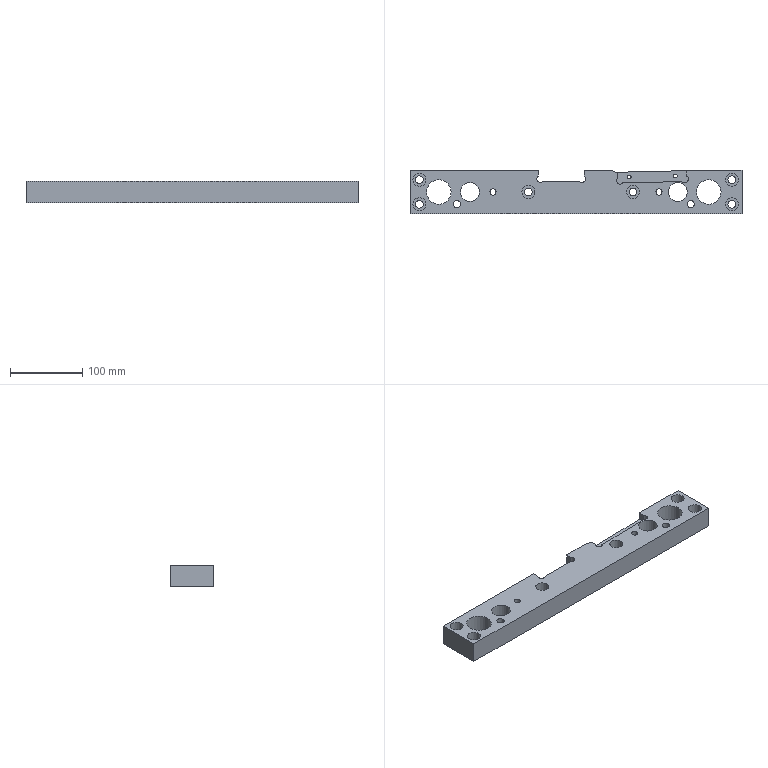Part | NX | features LIN_SOLID_COLOR 2 | 1 solid | 54 faces | box 460 x 60 x 30 mm | volume 649468 mm3 | cylinder 30 | plane 24 | commonest cylinder face diameters 11 x6 18 x6 10 x4 5.2 x2 8.5 x2 10.001 x2
STEP:
#1=CARTESIAN_POINT('',(659.328,-119.27,-12.));
#2=VERTEX_POINT('',#1);
#3=CARTESIAN_POINT('',(656.728,-119.27,-12.));
#4=DIRECTION('',(0.,0.,-1.));
#5=DIRECTION('',(1.,0.,0.));
#6=AXIS2_PLACEMENT_3D('',#3,#4,#5);
#7=CIRCLE('',#6,2.6);
#8=EDGE_CURVE('',#2,#2,#7,.T.);
#9=ORIENTED_EDGE('',*,*,#8,.T.);
#10=EDGE_LOOP('',(#9));
#11=FACE_BOUND('',#10,.T.);
#12=CARTESIAN_POINT('',(640.567,-112.648,-12.));
#13=VERTEX_POINT('',#12);
#14=CARTESIAN_POINT('',(736.541,-110.39,-12.));
#15=VERTEX_POINT('',#14);
#16=CARTESIAN_POINT('',(735.541,-110.413,-12.));
#17=DIRECTION('',(0.9997,0.02352,0.));
#18=VECTOR('',#17,1000.);
#19=LINE('',#16,#18);
#20=EDGE_CURVE('',#13,#15,#19,.T.);
#21=ORIENTED_EDGE('',*,*,#20,.F.);
#22=CARTESIAN_POINT('',(640.755,-120.607,-12.));
#23=VERTEX_POINT('',#22);
#24=CARTESIAN_POINT('',(640.732,-119.646,-12.));
#25=DIRECTION('',(0.02352,-0.9997,0.));
#26=VECTOR('',#25,1000.);
#27=LINE('',#24,#26);
#28=EDGE_CURVE('',#13,#23,#27,.T.);
#29=ORIENTED_EDGE('',*,*,#28,.T.);
#30=CARTESIAN_POINT('',(647.957,-127.478,-12.));
#31=VERTEX_POINT('',#30);
#32=CARTESIAN_POINT('',(644.026,-124.388,-12.));
#33=DIRECTION('',(0.,0.,1.));
#34=DIRECTION('',(1.,0.,0.));
#35=AXIS2_PLACEMENT_3D('',#32,#33,#34);
#36=CIRCLE('',#35,5.);
#37=EDGE_CURVE('',#23,#31,#36,.T.);
#38=ORIENTED_EDGE('',*,*,#37,.T.);
#39=CARTESIAN_POINT('',(729.857,-125.551,-12.));
#40=VERTEX_POINT('',#39);
#41=CARTESIAN_POINT('',(735.894,-125.409,-12.));
#42=DIRECTION('',(0.9997,0.02352,0.));
#43=VECTOR('',#42,1000.);
#44=LINE('',#41,#43);
#45=EDGE_CURVE('',#40,#31,#44,.F.);
#46=ORIENTED_EDGE('',*,*,#45,.F.);
#47=CARTESIAN_POINT('',(736.728,-118.349,-12.));
#48=VERTEX_POINT('',#47);
#49=CARTESIAN_POINT('',(733.638,-122.279,-12.));
#50=DIRECTION('',(0.,0.,1.));
#51=DIRECTION('',(1.,0.,0.));
#52=AXIS2_PLACEMENT_3D('',#49,#50,#51);
#53=CIRCLE('',#52,5.);
#54=EDGE_CURVE('',#40,#48,#53,.T.);
#55=ORIENTED_EDGE('',*,*,#54,.T.);
#56=CARTESIAN_POINT('',(736.705,-117.388,-12.));
#57=DIRECTION('',(0.02352,-0.9997,0.));
#58=VECTOR('',#57,1000.);
#59=LINE('',#56,#58);
#60=EDGE_CURVE('',#15,#48,#59,.T.);
#61=ORIENTED_EDGE('',*,*,#60,.F.);
#62=EDGE_LOOP('',(#21,#29,#38,#46,#55,#61));
#63=FACE_BOUND('',#62,.T.);
#64=CARTESIAN_POINT('',(723.31,-117.764,-12.));
#65=VERTEX_POINT('',#64);
#66=CARTESIAN_POINT('',(720.71,-117.764,-12.));
#67=DIRECTION('',(0.,0.,-1.));
#68=DIRECTION('',(1.,0.,0.));
#69=AXIS2_PLACEMENT_3D('',#66,#67,#68);
#70=CIRCLE('',#69,2.6);
#71=EDGE_CURVE('',#65,#65,#70,.T.);
#72=ORIENTED_EDGE('',*,*,#71,.T.);
#73=EDGE_LOOP('',(#72));
#74=FACE_BOUND('',#73,.T.);
#75=CARTESIAN_POINT('',(735.706,-117.411,-12.));
#76=DIRECTION('',(0.,0.,1.));
#77=DIRECTION('',(1.,0.,0.));
#78=AXIS2_PLACEMENT_3D('',#75,#76,#77);
#79=PLANE('',#78);
#80=ADVANCED_FACE('',(#11,#63,#74),#79,.T.);
#81=CARTESIAN_POINT('',(671.,-140.,-1.5));
#82=VERTEX_POINT('',#81);
#83=CARTESIAN_POINT('',(662.,-140.,-1.5));
#84=DIRECTION('',(0.,0.,1.));
#85=DIRECTION('',(1.,0.,0.));
#86=AXIS2_PLACEMENT_3D('',#83,#84,#85);
#87=CIRCLE('',#86,9.);
#88=EDGE_CURVE('',#82,#82,#87,.T.);
#89=ORIENTED_EDGE('',*,*,#88,.F.);
#90=EDGE_LOOP('',(#89));
#91=FACE_BOUND('',#90,.T.);
#92=CARTESIAN_POINT('',(410.,-140.,-1.5));
#93=VERTEX_POINT('',#92);
#94=CARTESIAN_POINT('',(393.,-140.,-1.5));
#95=DIRECTION('',(0.,0.,1.));
#96=DIRECTION('',(1.,0.,0.));
#97=AXIS2_PLACEMENT_3D('',#94,#95,#96);
#98=CIRCLE('',#97,17.);
#99=EDGE_CURVE('',#93,#93,#98,.T.);
#100=ORIENTED_EDGE('',*,*,#99,.F.);
#101=EDGE_LOOP('',(#100));
#102=FACE_BOUND('',#101,.T.);
#103=CARTESIAN_POINT('',(784.,-140.,-1.5));
#104=VERTEX_POINT('',#103);
#105=CARTESIAN_POINT('',(767.,-140.,-1.5));
#106=DIRECTION('',(0.,0.,1.));
#107=DIRECTION('',(1.,0.,0.));
#108=AXIS2_PLACEMENT_3D('',#105,#106,#107);
#109=CIRCLE('',#108,17.);
#110=EDGE_CURVE('',#104,#104,#109,.F.);
#111=ORIENTED_EDGE('',*,*,#110,.T.);
#112=EDGE_LOOP('',(#111));
#113=FACE_BOUND('',#112,.T.);
#114=CARTESIAN_POINT('',(375.,-157.,-1.5));
#115=VERTEX_POINT('',#114);
#116=CARTESIAN_POINT('',(366.,-157.,-1.5));
#117=DIRECTION('',(0.,0.,1.));
#118=DIRECTION('',(1.,0.,0.));
#119=AXIS2_PLACEMENT_3D('',#116,#117,#118);
#120=CIRCLE('',#119,9.);
#121=EDGE_CURVE('',#115,#115,#120,.T.);
#122=ORIENTED_EDGE('',*,*,#121,.F.);
#123=EDGE_LOOP('',(#122));
#124=FACE_BOUND('',#123,.T.);
#125=CARTESIAN_POINT('',(375.,-123.,-1.5));
#126=VERTEX_POINT('',#125);
#127=CARTESIAN_POINT('',(366.,-123.,-1.5));
#128=DIRECTION('',(0.,0.,1.));
#129=DIRECTION('',(1.,0.,0.));
#130=AXIS2_PLACEMENT_3D('',#127,#128,#129);
#131=CIRCLE('',#130,9.);
#132=EDGE_CURVE('',#126,#126,#131,.T.);
#133=ORIENTED_EDGE('',*,*,#132,.F.);
#134=EDGE_LOOP('',(#133));
#135=FACE_BOUND('',#134,.T.);
#136=CARTESIAN_POINT('',(423.004,-157.,-1.5));
#137=VERTEX_POINT('',#136);
#138=CARTESIAN_POINT('',(418.003,-157.,-1.5));
#139=DIRECTION('',(0.,0.,1.));
#140=DIRECTION('',(1.,0.,0.));
#141=AXIS2_PLACEMENT_3D('',#138,#139,#140);
#142=CIRCLE('',#141,5.);
#143=EDGE_CURVE('',#137,#137,#142,.T.);
#144=ORIENTED_EDGE('',*,*,#143,.F.);
#145=EDGE_LOOP('',(#144));
#146=FACE_BOUND('',#145,.T.);
#147=CARTESIAN_POINT('',(526.,-140.,-1.5));
#148=VERTEX_POINT('',#147);
#149=CARTESIAN_POINT('',(517.,-140.,-1.5));
#150=DIRECTION('',(0.,0.,1.));
#151=DIRECTION('',(1.,0.,0.));
#152=AXIS2_PLACEMENT_3D('',#149,#150,#151);
#153=CIRCLE('',#152,9.);
#154=EDGE_CURVE('',#148,#148,#153,.T.);
#155=ORIENTED_EDGE('',*,*,#154,.F.);
#156=EDGE_LOOP('',(#155));
#157=FACE_BOUND('',#156,.T.);
#158=CARTESIAN_POINT('',(746.997,-157.,-1.5));
#159=VERTEX_POINT('',#158);
#160=CARTESIAN_POINT('',(741.997,-157.,-1.5));
#161=DIRECTION('',(0.,0.,1.));
#162=DIRECTION('',(1.,0.,0.));
#163=AXIS2_PLACEMENT_3D('',#160,#161,#162);
#164=CIRCLE('',#163,5.);
#165=EDGE_CURVE('',#159,#159,#164,.T.);
#166=ORIENTED_EDGE('',*,*,#165,.F.);
#167=EDGE_LOOP('',(#166));
#168=FACE_BOUND('',#167,.T.);
#169=CARTESIAN_POINT('',(808.,-157.,-1.5));
#170=VERTEX_POINT('',#169);
#171=CARTESIAN_POINT('',(799.,-157.,-1.5));
#172=DIRECTION('',(0.,0.,1.));
#173=DIRECTION('',(1.,0.,0.));
#174=AXIS2_PLACEMENT_3D('',#171,#172,#173);
#175=CIRCLE('',#174,9.);
#176=EDGE_CURVE('',#170,#170,#175,.T.);
#177=ORIENTED_EDGE('',*,*,#176,.F.);
#178=EDGE_LOOP('',(#177));
#179=FACE_BOUND('',#178,.T.);
#180=CARTESIAN_POINT('',(808.,-123.,-1.5));
#181=VERTEX_POINT('',#180);
#182=CARTESIAN_POINT('',(799.,-123.,-1.5));
#183=DIRECTION('',(0.,0.,1.));
#184=DIRECTION('',(1.,0.,0.));
#185=AXIS2_PLACEMENT_3D('',#182,#183,#184);
#186=CIRCLE('',#185,9.);
#187=EDGE_CURVE('',#181,#181,#186,.T.);
#188=ORIENTED_EDGE('',*,*,#187,.F.);
#189=EDGE_LOOP('',(#188));
#190=FACE_BOUND('',#189,.T.);
#191=CARTESIAN_POINT('',(737.,-140.,-1.5));
#192=VERTEX_POINT('',#191);
#193=CARTESIAN_POINT('',(724.,-140.,-1.5));
#194=DIRECTION('',(0.,0.,1.));
#195=DIRECTION('',(1.,0.,0.));
#196=AXIS2_PLACEMENT_3D('',#193,#194,#195);
#197=CIRCLE('',#196,13.);
#198=EDGE_CURVE('',#192,#192,#197,.T.);
#199=ORIENTED_EDGE('',*,*,#198,.F.);
#200=EDGE_LOOP('',(#199));
#201=FACE_BOUND('',#200,.T.);
#202=CARTESIAN_POINT('',(449.,-140.,-1.5));
#203=VERTEX_POINT('',#202);
#204=CARTESIAN_POINT('',(436.,-140.,-1.5));
#205=DIRECTION('',(0.,0.,1.));
#206=DIRECTION('',(1.,0.,0.));
#207=AXIS2_PLACEMENT_3D('',#204,#205,#206);
#208=CIRCLE('',#207,13.);
#209=EDGE_CURVE('',#203,#203,#208,.F.);
#210=ORIENTED_EDGE('',*,*,#209,.T.);
#211=EDGE_LOOP('',(#210));
#212=FACE_BOUND('',#211,.T.);
#213=CARTESIAN_POINT('',(587.461,-125.,-1.5));
#214=VERTEX_POINT('',#213);
#215=CARTESIAN_POINT('',(537.539,-125.,-1.5));
#216=VERTEX_POINT('',#215);
#217=CARTESIAN_POINT('',(645.,-125.,-1.5));
#218=DIRECTION('',(-1.,0.,0.));
#219=VECTOR('',#218,1000.);
#220=LINE('',#217,#219);
#221=EDGE_CURVE('',#214,#216,#220,.T.);
#222=ORIENTED_EDGE('',*,*,#221,.T.);
#223=CARTESIAN_POINT('',(530.5,-117.961,-1.5));
#224=VERTEX_POINT('',#223);
#225=CARTESIAN_POINT('',(533.682,-121.818,-1.5));
#226=DIRECTION('',(0.,0.,-1.));
#227=DIRECTION('',(1.,0.,0.));
#228=AXIS2_PLACEMENT_3D('',#225,#226,#227);
#229=CIRCLE('',#228,5.);
#230=EDGE_CURVE('',#216,#224,#229,.T.);
#231=ORIENTED_EDGE('',*,*,#230,.T.);
#232=CARTESIAN_POINT('',(530.5,-110.,-1.5));
#233=VERTEX_POINT('',#232);
#234=CARTESIAN_POINT('',(530.5,0.,-1.5));
#235=DIRECTION('',(0.,1.,0.));
#236=VECTOR('',#235,1000.);
#237=LINE('',#234,#236);
#238=EDGE_CURVE('',#224,#233,#237,.T.);
#239=ORIENTED_EDGE('',*,*,#238,.T.);
#240=CARTESIAN_POINT('',(353.,-110.,-1.5));
#241=VERTEX_POINT('',#240);
#242=CARTESIAN_POINT('',(667.,-110.,-1.5));
#243=DIRECTION('',(-1.,0.,0.));
#244=VECTOR('',#243,1000.);
#245=LINE('',#242,#244);
#246=EDGE_CURVE('',#241,#233,#245,.F.);
#247=ORIENTED_EDGE('',*,*,#246,.F.);
#248=CARTESIAN_POINT('',(353.,-170.,-1.5));
#249=VERTEX_POINT('',#248);
#250=CARTESIAN_POINT('',(353.,-30.,-1.5));
#251=DIRECTION('',(0.,1.,0.));
#252=VECTOR('',#251,1000.);
#253=LINE('',#250,#252);
#254=EDGE_CURVE('',#249,#241,#253,.T.);
#255=ORIENTED_EDGE('',*,*,#254,.F.);
#256=CARTESIAN_POINT('',(813.,-170.,-1.5));
#257=VERTEX_POINT('',#256);
#258=CARTESIAN_POINT('',(667.,-170.,-1.5));
#259=DIRECTION('',(1.,0.,0.));
#260=VECTOR('',#259,1000.);
#261=LINE('',#258,#260);
#262=EDGE_CURVE('',#257,#249,#261,.F.);
#263=ORIENTED_EDGE('',*,*,#262,.F.);
#264=CARTESIAN_POINT('',(813.,-110.,-1.5));
#265=VERTEX_POINT('',#264);
#266=CARTESIAN_POINT('',(813.,-173.255,-1.5));
#267=DIRECTION('',(0.,1.,0.));
#268=VECTOR('',#267,1000.);
#269=LINE('',#266,#268);
#270=EDGE_CURVE('',#257,#265,#269,.T.);
#271=ORIENTED_EDGE('',*,*,#270,.T.);
#272=CARTESIAN_POINT('',(739.752,-110.,-1.5));
#273=VERTEX_POINT('',#272);
#274=CARTESIAN_POINT('',(667.,-110.,-1.5));
#275=DIRECTION('',(-1.,0.,0.));
#276=VECTOR('',#275,1000.);
#277=LINE('',#274,#276);
#278=EDGE_CURVE('',#273,#265,#277,.F.);
#279=ORIENTED_EDGE('',*,*,#278,.F.);
#280=CARTESIAN_POINT('',(737.54,-110.366,-1.5));
#281=VERTEX_POINT('',#280);
#282=CARTESIAN_POINT('',(737.352,-102.368,-1.5));
#283=DIRECTION('',(0.,0.,1.));
#284=DIRECTION('',(1.,0.,0.));
#285=AXIS2_PLACEMENT_3D('',#282,#283,#284);
#286=CIRCLE('',#285,8.);
#287=EDGE_CURVE('',#281,#273,#286,.T.);
#288=ORIENTED_EDGE('',*,*,#287,.F.);
#289=CARTESIAN_POINT('',(736.541,-110.39,-1.5));
#290=VERTEX_POINT('',#289);
#291=CARTESIAN_POINT('',(628.78,-112.925,-1.5));
#292=DIRECTION('',(0.9997,0.02352,0.));
#293=VECTOR('',#292,1000.);
#294=LINE('',#291,#293);
#295=EDGE_CURVE('',#290,#281,#294,.T.);
#296=ORIENTED_EDGE('',*,*,#295,.F.);
#297=CARTESIAN_POINT('',(736.728,-118.349,-1.5));
#298=VERTEX_POINT('',#297);
#299=CARTESIAN_POINT('',(737.96,-170.72,-1.5));
#300=DIRECTION('',(0.02352,-0.9997,0.));
#301=VECTOR('',#300,1000.);
#302=LINE('',#299,#301);
#303=EDGE_CURVE('',#290,#298,#302,.T.);
#304=ORIENTED_EDGE('',*,*,#303,.T.);
#305=CARTESIAN_POINT('',(729.857,-125.551,-1.5));
#306=VERTEX_POINT('',#305);
#307=CARTESIAN_POINT('',(733.638,-122.279,-1.5));
#308=DIRECTION('',(0.,0.,1.));
#309=DIRECTION('',(1.,0.,0.));
#310=AXIS2_PLACEMENT_3D('',#307,#308,#309);
#311=CIRCLE('',#310,5.);
#312=EDGE_CURVE('',#306,#298,#311,.T.);
#313=ORIENTED_EDGE('',*,*,#312,.F.);
#314=CARTESIAN_POINT('',(647.957,-127.478,-1.5));
#315=VERTEX_POINT('',#314);
#316=CARTESIAN_POINT('',(629.133,-127.921,-1.5));
#317=DIRECTION('',(0.9997,0.02352,0.));
#318=VECTOR('',#317,1000.);
#319=LINE('',#316,#318);
#320=EDGE_CURVE('',#315,#306,#319,.T.);
#321=ORIENTED_EDGE('',*,*,#320,.F.);
#322=CARTESIAN_POINT('',(640.755,-120.607,-1.5));
#323=VERTEX_POINT('',#322);
#324=CARTESIAN_POINT('',(644.026,-124.388,-1.5));
#325=DIRECTION('',(0.,0.,1.));
#326=DIRECTION('',(1.,0.,0.));
#327=AXIS2_PLACEMENT_3D('',#324,#325,#326);
#328=CIRCLE('',#327,5.);
#329=EDGE_CURVE('',#323,#315,#328,.T.);
#330=ORIENTED_EDGE('',*,*,#329,.F.);
#331=CARTESIAN_POINT('',(640.567,-112.648,-1.5));
#332=VERTEX_POINT('',#331);
#333=CARTESIAN_POINT('',(641.987,-172.978,-1.5));
#334=DIRECTION('',(-0.02352,0.9997,0.));
#335=VECTOR('',#334,1000.);
#336=LINE('',#333,#335);
#337=EDGE_CURVE('',#323,#332,#336,.T.);
#338=ORIENTED_EDGE('',*,*,#337,.T.);
#339=CARTESIAN_POINT('',(639.568,-112.671,-1.5));
#340=VERTEX_POINT('',#339);
#341=CARTESIAN_POINT('',(628.78,-112.925,-1.5));
#342=DIRECTION('',(0.9997,0.02352,0.));
#343=VECTOR('',#342,1000.);
#344=LINE('',#341,#343);
#345=EDGE_CURVE('',#340,#332,#344,.T.);
#346=ORIENTED_EDGE('',*,*,#345,.F.);
#347=CARTESIAN_POINT('',(633.41,-110.,-1.5));
#348=VERTEX_POINT('',#347);
#349=CARTESIAN_POINT('',(639.379,-104.674,-1.5));
#350=DIRECTION('',(0.,0.,1.));
#351=DIRECTION('',(1.,0.,0.));
#352=AXIS2_PLACEMENT_3D('',#349,#350,#351);
#353=CIRCLE('',#352,8.);
#354=EDGE_CURVE('',#348,#340,#353,.T.);
#355=ORIENTED_EDGE('',*,*,#354,.F.);
#356=CARTESIAN_POINT('',(594.5,-110.,-1.5));
#357=VERTEX_POINT('',#356);
#358=CARTESIAN_POINT('',(667.,-110.,-1.5));
#359=DIRECTION('',(-1.,0.,0.));
#360=VECTOR('',#359,1000.);
#361=LINE('',#358,#360);
#362=EDGE_CURVE('',#357,#348,#361,.F.);
#363=ORIENTED_EDGE('',*,*,#362,.F.);
#364=CARTESIAN_POINT('',(594.5,-117.961,-1.5));
#365=VERTEX_POINT('',#364);
#366=CARTESIAN_POINT('',(594.5,-173.255,-1.5));
#367=DIRECTION('',(0.,-1.,0.));
#368=VECTOR('',#367,1000.);
#369=LINE('',#366,#368);
#370=EDGE_CURVE('',#357,#365,#369,.T.);
#371=ORIENTED_EDGE('',*,*,#370,.T.);
#372=CARTESIAN_POINT('',(591.318,-121.818,-1.5));
#373=DIRECTION('',(0.,0.,-1.));
#374=DIRECTION('',(1.,0.,0.));
#375=AXIS2_PLACEMENT_3D('',#372,#373,#374);
#376=CIRCLE('',#375,5.);
#377=EDGE_CURVE('',#365,#214,#376,.T.);
#378=ORIENTED_EDGE('',*,*,#377,.T.);
#379=EDGE_LOOP('',(#222,#231,#239,#247,#255,#263,#271,#279,#288,#296,#304,#313,#321,#330,#338,#346,#355,#363,#371,#378));
#380=FACE_BOUND('',#379,.T.);
#381=CARTESIAN_POINT('',(472.25,-140.,-1.5));
#382=VERTEX_POINT('',#381);
#383=CARTESIAN_POINT('',(468.,-140.,-1.5));
#384=DIRECTION('',(0.,0.,1.));
#385=DIRECTION('',(1.,0.,0.));
#386=AXIS2_PLACEMENT_3D('',#383,#384,#385);
#387=CIRCLE('',#386,4.25);
#388=EDGE_CURVE('',#382,#382,#387,.T.);
#389=ORIENTED_EDGE('',*,*,#388,.F.);
#390=EDGE_LOOP('',(#389));
#391=FACE_BOUND('',#390,.T.);
#392=CARTESIAN_POINT('',(693.75,-140.,-1.5));
#393=VERTEX_POINT('',#392);
#394=CARTESIAN_POINT('',(698.,-140.,-1.5));
#395=DIRECTION('',(0.,0.,-1.));
#396=DIRECTION('',(-1.,0.,0.));
#397=AXIS2_PLACEMENT_3D('',#394,#395,#396);
#398=CIRCLE('',#397,4.25);
#399=EDGE_CURVE('',#393,#393,#398,.T.);
#400=ORIENTED_EDGE('',*,*,#399,.T.);
#401=EDGE_LOOP('',(#400));
#402=FACE_BOUND('',#401,.T.);
#403=CARTESIAN_POINT('',(630.2,-173.255,-1.5));
#404=DIRECTION('',(0.,0.,1.));
#405=DIRECTION('',(1.,0.,0.));
#406=AXIS2_PLACEMENT_3D('',#403,#404,#405);
#407=PLANE('',#406);
#408=ADVANCED_FACE('',(#91,#102,#113,#124,#135,#146,#157,#168,#179,#190,#201,#212,#380,#391,#402),#407,.T.);
#409=CARTESIAN_POINT('',(718.11,-117.764,-31.5));
#410=VERTEX_POINT('',#409);
#411=CARTESIAN_POINT('',(720.71,-117.764,-31.5));
#412=DIRECTION('',(0.,0.,-1.));
#413=DIRECTION('',(-1.,0.,0.));
#414=AXIS2_PLACEMENT_3D('',#411,#412,#413);
#415=CIRCLE('',#414,2.6);
#416=EDGE_CURVE('',#410,#410,#415,.T.);
#417=ORIENTED_EDGE('',*,*,#416,.F.);
#418=EDGE_LOOP('',(#417));
#419=FACE_BOUND('',#418,.T.);
#420=CARTESIAN_POINT('',(654.128,-119.27,-31.5));
#421=VERTEX_POINT('',#420);
#422=CARTESIAN_POINT('',(656.728,-119.27,-31.5));
#423=DIRECTION('',(0.,0.,-1.));
#424=DIRECTION('',(-1.,0.,0.));
#425=AXIS2_PLACEMENT_3D('',#422,#423,#424);
#426=CIRCLE('',#425,2.6);
#427=EDGE_CURVE('',#421,#421,#426,.T.);
#428=ORIENTED_EDGE('',*,*,#427,.F.);
#429=EDGE_LOOP('',(#428));
#430=FACE_BOUND('',#429,.T.);
#431=CARTESIAN_POINT('',(693.75,-140.,-31.5));
#432=VERTEX_POINT('',#431);
#433=CARTESIAN_POINT('',(698.,-140.,-31.5));
#434=DIRECTION('',(0.,0.,-1.));
#435=DIRECTION('',(-1.,0.,0.));
#436=AXIS2_PLACEMENT_3D('',#433,#434,#435);
#437=CIRCLE('',#436,4.25);
#438=EDGE_CURVE('',#432,#432,#437,.T.);
#439=ORIENTED_EDGE('',*,*,#438,.F.);
#440=EDGE_LOOP('',(#439));
#441=FACE_BOUND('',#440,.T.);
#442=CARTESIAN_POINT('',(463.75,-140.,-31.5));
#443=VERTEX_POINT('',#442);
#444=CARTESIAN_POINT('',(468.,-140.,-31.5));
#445=DIRECTION('',(0.,0.,-1.));
#446=DIRECTION('',(-1.,0.,0.));
#447=AXIS2_PLACEMENT_3D('',#444,#445,#446);
#448=CIRCLE('',#447,4.25);
#449=EDGE_CURVE('',#443,#443,#448,.T.);
#450=ORIENTED_EDGE('',*,*,#449,.F.);
#451=EDGE_LOOP('',(#450));
#452=FACE_BOUND('',#451,.T.);
#453=CARTESIAN_POINT('',(423.,-140.,-31.5));
#454=VERTEX_POINT('',#453);
#455=CARTESIAN_POINT('',(436.,-140.,-31.5));
#456=DIRECTION('',(0.,0.,-1.));
#457=DIRECTION('',(-1.,0.,0.));
#458=AXIS2_PLACEMENT_3D('',#455,#456,#457);
#459=CIRCLE('',#458,13.);
#460=EDGE_CURVE('',#454,#454,#459,.F.);
#461=ORIENTED_EDGE('',*,*,#460,.T.);
#462=EDGE_LOOP('',(#461));
#463=FACE_BOUND('',#462,.T.);
#464=CARTESIAN_POINT('',(711.,-140.,-31.5));
#465=VERTEX_POINT('',#464);
#466=CARTESIAN_POINT('',(724.,-140.,-31.5));
#467=DIRECTION('',(0.,0.,-1.));
#468=DIRECTION('',(-1.,0.,0.));
#469=AXIS2_PLACEMENT_3D('',#466,#467,#468);
#470=CIRCLE('',#469,13.);
#471=EDGE_CURVE('',#465,#465,#470,.T.);
#472=ORIENTED_EDGE('',*,*,#471,.F.);
#473=EDGE_LOOP('',(#472));
#474=FACE_BOUND('',#473,.T.);
#475=CARTESIAN_POINT('',(793.5,-123.,-31.5));
#476=VERTEX_POINT('',#475);
#477=CARTESIAN_POINT('',(799.,-123.,-31.5));
#478=DIRECTION('',(0.,0.,-1.));
#479=DIRECTION('',(-1.,0.,0.));
#480=AXIS2_PLACEMENT_3D('',#477,#478,#479);
#481=CIRCLE('',#480,5.5);
#482=EDGE_CURVE('',#476,#476,#481,.T.);
#483=ORIENTED_EDGE('',*,*,#482,.F.);
#484=EDGE_LOOP('',(#483));
#485=FACE_BOUND('',#484,.T.);
#486=CARTESIAN_POINT('',(793.5,-157.,-31.5));
#487=VERTEX_POINT('',#486);
#488=CARTESIAN_POINT('',(799.,-157.,-31.5));
#489=DIRECTION('',(0.,0.,-1.));
#490=DIRECTION('',(-1.,0.,0.));
#491=AXIS2_PLACEMENT_3D('',#488,#489,#490);
#492=CIRCLE('',#491,5.5);
#493=EDGE_CURVE('',#487,#487,#492,.T.);
#494=ORIENTED_EDGE('',*,*,#493,.F.);
#495=EDGE_LOOP('',(#494));
#496=FACE_BOUND('',#495,.T.);
#497=CARTESIAN_POINT('',(736.996,-157.,-31.5));
#498=VERTEX_POINT('',#497);
#499=CARTESIAN_POINT('',(741.997,-157.,-31.5));
#500=DIRECTION('',(0.,0.,-1.));
#501=DIRECTION('',(-1.,0.,0.));
#502=AXIS2_PLACEMENT_3D('',#499,#500,#501);
#503=CIRCLE('',#502,5.);
#504=EDGE_CURVE('',#498,#498,#503,.T.);
#505=ORIENTED_EDGE('',*,*,#504,.F.);
#506=EDGE_LOOP('',(#505));
#507=FACE_BOUND('',#506,.T.);
#508=CARTESIAN_POINT('',(511.5,-140.,-31.5));
#509=VERTEX_POINT('',#508);
#510=CARTESIAN_POINT('',(517.,-140.,-31.5));
#511=DIRECTION('',(0.,0.,-1.));
#512=DIRECTION('',(-1.,0.,0.));
#513=AXIS2_PLACEMENT_3D('',#510,#511,#512);
#514=CIRCLE('',#513,5.5);
#515=EDGE_CURVE('',#509,#509,#514,.T.);
#516=ORIENTED_EDGE('',*,*,#515,.F.);
#517=EDGE_LOOP('',(#516));
#518=FACE_BOUND('',#517,.T.);
#519=CARTESIAN_POINT('',(374.,-140.,-31.5));
#520=VERTEX_POINT('',#519);
#521=CARTESIAN_POINT('',(393.,-140.,-31.5));
#522=DIRECTION('',(0.,0.,-1.));
#523=DIRECTION('',(-1.,0.,0.));
#524=AXIS2_PLACEMENT_3D('',#521,#522,#523);
#525=CIRCLE('',#524,19.);
#526=EDGE_CURVE('',#520,#520,#525,.F.);
#527=ORIENTED_EDGE('',*,*,#526,.T.);
#528=EDGE_LOOP('',(#527));
#529=FACE_BOUND('',#528,.T.);
#530=CARTESIAN_POINT('',(748.,-140.,-31.5));
#531=VERTEX_POINT('',#530);
#532=CARTESIAN_POINT('',(767.,-140.,-31.5));
#533=DIRECTION('',(0.,0.,-1.));
#534=DIRECTION('',(-1.,0.,0.));
#535=AXIS2_PLACEMENT_3D('',#532,#533,#534);
#536=CIRCLE('',#535,19.);
#537=EDGE_CURVE('',#531,#531,#536,.T.);
#538=ORIENTED_EDGE('',*,*,#537,.F.);
#539=EDGE_LOOP('',(#538));
#540=FACE_BOUND('',#539,.T.);
#541=CARTESIAN_POINT('',(360.5,-157.,-31.5));
#542=VERTEX_POINT('',#541);
#543=CARTESIAN_POINT('',(366.,-157.,-31.5));
#544=DIRECTION('',(0.,0.,-1.));
#545=DIRECTION('',(-1.,0.,0.));
#546=AXIS2_PLACEMENT_3D('',#543,#544,#545);
#547=CIRCLE('',#546,5.5);
#548=EDGE_CURVE('',#542,#542,#547,.T.);
#549=ORIENTED_EDGE('',*,*,#548,.F.);
#550=EDGE_LOOP('',(#549));
#551=FACE_BOUND('',#550,.T.);
#552=CARTESIAN_POINT('',(360.5,-123.,-31.5));
#553=VERTEX_POINT('',#552);
#554=CARTESIAN_POINT('',(366.,-123.,-31.5));
#555=DIRECTION('',(0.,0.,-1.));
#556=DIRECTION('',(-1.,0.,0.));
#557=AXIS2_PLACEMENT_3D('',#554,#555,#556);
#558=CIRCLE('',#557,5.5);
#559=EDGE_CURVE('',#553,#553,#558,.T.);
#560=ORIENTED_EDGE('',*,*,#559,.F.);
#561=EDGE_LOOP('',(#560));
#562=FACE_BOUND('',#561,.T.);
#563=CARTESIAN_POINT('',(413.003,-157.,-31.5));
#564=VERTEX_POINT('',#563);
#565=CARTESIAN_POINT('',(418.003,-157.,-31.5));
#566=DIRECTION('',(0.,0.,-1.));
#567=DIRECTION('',(-1.,0.,0.));
#568=AXIS2_PLACEMENT_3D('',#565,#566,#567);
#569=CIRCLE('',#568,5.);
#570=EDGE_CURVE('',#564,#564,#569,.F.);
#571=ORIENTED_EDGE('',*,*,#570,.T.);
#572=EDGE_LOOP('',(#571));
#573=FACE_BOUND('',#572,.T.);
#574=CARTESIAN_POINT('',(656.5,-140.,-31.5));
#575=VERTEX_POINT('',#574);
#576=CARTESIAN_POINT('',(662.,-140.,-31.5));
#577=DIRECTION('',(0.,0.,-1.));
#578=DIRECTION('',(-1.,0.,0.));
#579=AXIS2_PLACEMENT_3D('',#576,#577,#578);
#580=CIRCLE('',#579,5.5);
#581=EDGE_CURVE('',#575,#575,#580,.T.);
#582=ORIENTED_EDGE('',*,*,#581,.F.);
#583=EDGE_LOOP('',(#582));
#584=FACE_BOUND('',#583,.T.);
#585=CARTESIAN_POINT('',(530.5,-110.,-31.5));
#586=VERTEX_POINT('',#585);
#587=CARTESIAN_POINT('',(530.5,-117.961,-31.5));
#588=VERTEX_POINT('',#587);
#589=CARTESIAN_POINT('',(530.5,0.,-31.5));
#590=DIRECTION('',(0.,-1.,0.));
#591=VECTOR('',#590,1000.);
#592=LINE('',#589,#591);
#593=EDGE_CURVE('',#586,#588,#592,.T.);
#594=ORIENTED_EDGE('',*,*,#593,.T.);
#595=CARTESIAN_POINT('',(537.539,-125.,-31.5));
#596=VERTEX_POINT('',#595);
#597=CARTESIAN_POINT('',(533.682,-121.818,-31.5));
#598=DIRECTION('',(0.,0.,1.));
#599=DIRECTION('',(1.,0.,0.));
#600=AXIS2_PLACEMENT_3D('',#597,#598,#599);
#601=CIRCLE('',#600,5.);
#602=EDGE_CURVE('',#588,#596,#601,.T.);
#603=ORIENTED_EDGE('',*,*,#602,.T.);
#604=CARTESIAN_POINT('',(587.461,-125.,-31.5));
#605=VERTEX_POINT('',#604);
#606=CARTESIAN_POINT('',(645.,-125.,-31.5));
#607=DIRECTION('',(1.,0.,0.));
#608=VECTOR('',#607,1000.);
#609=LINE('',#606,#608);
#610=EDGE_CURVE('',#596,#605,#609,.T.);
#611=ORIENTED_EDGE('',*,*,#610,.T.);
#612=CARTESIAN_POINT('',(594.5,-117.961,-31.5));
#613=VERTEX_POINT('',#612);
#614=CARTESIAN_POINT('',(591.318,-121.818,-31.5));
#615=DIRECTION('',(0.,0.,1.));
#616=DIRECTION('',(1.,0.,0.));
#617=AXIS2_PLACEMENT_3D('',#614,#615,#616);
#618=CIRCLE('',#617,5.);
#619=EDGE_CURVE('',#605,#613,#618,.T.);
#620=ORIENTED_EDGE('',*,*,#619,.T.);
#621=CARTESIAN_POINT('',(594.5,-110.,-31.5));
#622=VERTEX_POINT('',#621);
#623=CARTESIAN_POINT('',(594.5,-140.,-31.5));
#624=DIRECTION('',(0.,1.,0.));
#625=VECTOR('',#624,1000.);
#626=LINE('',#623,#625);
#627=EDGE_CURVE('',#613,#622,#626,.T.);
#628=ORIENTED_EDGE('',*,*,#627,.T.);
#629=CARTESIAN_POINT('',(633.41,-110.,-31.5));
#630=VERTEX_POINT('',#629);
#631=CARTESIAN_POINT('',(667.,-110.,-31.5));
#632=DIRECTION('',(1.,0.,0.));
#633=VECTOR('',#632,1000.);
#634=LINE('',#631,#633);
#635=EDGE_CURVE('',#630,#622,#634,.F.);
#636=ORIENTED_EDGE('',*,*,#635,.F.);
#637=CARTESIAN_POINT('',(639.568,-112.671,-31.5));
#638=VERTEX_POINT('',#637);
#639=CARTESIAN_POINT('',(639.379,-104.674,-31.5));
#640=DIRECTION('',(0.,0.,-1.));
#641=DIRECTION('',(-1.,0.,0.));
#642=AXIS2_PLACEMENT_3D('',#639,#640,#641);
#643=CIRCLE('',#642,8.);
#644=EDGE_CURVE('',#638,#630,#643,.T.);
#645=ORIENTED_EDGE('',*,*,#644,.F.);
#646=CARTESIAN_POINT('',(737.54,-110.366,-31.5));
#647=VERTEX_POINT('',#646);
#648=CARTESIAN_POINT('',(666.342,-112.041,-31.5));
#649=DIRECTION('',(-0.9997,-0.02352,0.));
#650=VECTOR('',#649,1000.);
#651=LINE('',#648,#650);
#652=EDGE_CURVE('',#647,#638,#651,.T.);
#653=ORIENTED_EDGE('',*,*,#652,.F.);
#654=CARTESIAN_POINT('',(739.752,-110.,-31.5));
#655=VERTEX_POINT('',#654);
#656=CARTESIAN_POINT('',(737.352,-102.368,-31.5));
#657=DIRECTION('',(0.,0.,-1.));
#658=DIRECTION('',(-1.,0.,0.));
#659=AXIS2_PLACEMENT_3D('',#656,#657,#658);
#660=CIRCLE('',#659,8.);
#661=EDGE_CURVE('',#655,#647,#660,.T.);
#662=ORIENTED_EDGE('',*,*,#661,.F.);
#663=CARTESIAN_POINT('',(813.,-110.,-31.5));
#664=VERTEX_POINT('',#663);
#665=CARTESIAN_POINT('',(667.,-110.,-31.5));
#666=DIRECTION('',(1.,0.,0.));
#667=VECTOR('',#666,1000.);
#668=LINE('',#665,#667);
#669=EDGE_CURVE('',#664,#655,#668,.F.);
#670=ORIENTED_EDGE('',*,*,#669,.F.);
#671=CARTESIAN_POINT('',(813.,-170.,-31.5));
#672=VERTEX_POINT('',#671);
#673=CARTESIAN_POINT('',(813.,-140.,-31.5));
#674=DIRECTION('',(0.,-1.,0.));
#675=VECTOR('',#674,1000.);
#676=LINE('',#673,#675);
#677=EDGE_CURVE('',#664,#672,#676,.T.);
#678=ORIENTED_EDGE('',*,*,#677,.T.);
#679=CARTESIAN_POINT('',(353.,-170.,-31.5));
#680=VERTEX_POINT('',#679);
#681=CARTESIAN_POINT('',(667.,-170.,-31.5));
#682=DIRECTION('',(-1.,0.,0.));
#683=VECTOR('',#682,1000.);
#684=LINE('',#681,#683);
#685=EDGE_CURVE('',#680,#672,#684,.F.);
#686=ORIENTED_EDGE('',*,*,#685,.F.);
#687=CARTESIAN_POINT('',(353.,-110.,-31.5));
#688=VERTEX_POINT('',#687);
#689=CARTESIAN_POINT('',(353.,-30.,-31.5));
#690=DIRECTION('',(0.,-1.,0.));
#691=VECTOR('',#690,1000.);
#692=LINE('',#689,#691);
#693=EDGE_CURVE('',#688,#680,#692,.T.);
#694=ORIENTED_EDGE('',*,*,#693,.F.);
#695=CARTESIAN_POINT('',(667.,-110.,-31.5));
#696=DIRECTION('',(1.,0.,0.));
#697=VECTOR('',#696,1000.);
#698=LINE('',#695,#697);
#699=EDGE_CURVE('',#586,#688,#698,.F.);
#700=ORIENTED_EDGE('',*,*,#699,.F.);
#701=EDGE_LOOP('',(#594,#603,#611,#620,#628,#636,#645,#653,#662,#670,#678,#686,#694,#700));
#702=FACE_BOUND('',#701,.T.);
#703=CARTESIAN_POINT('',(667.,-140.,-31.5));
#704=DIRECTION('',(0.,0.,-1.));
#705=DIRECTION('',(1.,0.,0.));
#706=AXIS2_PLACEMENT_3D('',#703,#704,#705);
#707=PLANE('',#706);
#708=ADVANCED_FACE('',(#419,#430,#441,#452,#463,#474,#485,#496,#507,#518,#529,#540,#551,#562,#573,#584,#702),#707,.T.);
#709=ORIENTED_EDGE('',*,*,#635,.T.);
#710=CARTESIAN_POINT('',(594.5,-110.,-41.5));
#711=DIRECTION('',(0.,0.,1.));
#712=VECTOR('',#711,1000.);
#713=LINE('',#710,#712);
#714=EDGE_CURVE('',#622,#357,#713,.T.);
#715=ORIENTED_EDGE('',*,*,#714,.T.);
#716=ORIENTED_EDGE('',*,*,#362,.T.);
#717=CARTESIAN_POINT('',(633.41,-110.,70.));
#718=DIRECTION('',(0.,0.,1.));
#719=VECTOR('',#718,1000.);
#720=LINE('',#717,#719);
#721=EDGE_CURVE('',#630,#348,#720,.T.);
#722=ORIENTED_EDGE('',*,*,#721,.F.);
#723=EDGE_LOOP('',(#709,#715,#716,#722));
#724=FACE_BOUND('',#723,.T.);
#725=CARTESIAN_POINT('',(667.,-110.,-41.5));
#726=DIRECTION('',(0.,1.,0.));
#727=DIRECTION('',(0.,0.,1.));
#728=AXIS2_PLACEMENT_3D('',#725,#726,#727);
#729=PLANE('',#728);
#730=ADVANCED_FACE('',(#724),#729,.T.);
#731=CARTESIAN_POINT('',(530.5,-110.,-41.5));
#732=DIRECTION('',(0.,0.,1.));
#733=VECTOR('',#732,1000.);
#734=LINE('',#731,#733);
#735=EDGE_CURVE('',#586,#233,#734,.T.);
#736=ORIENTED_EDGE('',*,*,#735,.F.);
#737=ORIENTED_EDGE('',*,*,#699,.T.);
#738=CARTESIAN_POINT('',(353.,-110.,-41.5));
#739=DIRECTION('',(0.,0.,1.));
#740=VECTOR('',#739,1000.);
#741=LINE('',#738,#740);
#742=EDGE_CURVE('',#688,#241,#741,.T.);
#743=ORIENTED_EDGE('',*,*,#742,.T.);
#744=ORIENTED_EDGE('',*,*,#246,.T.);
#745=EDGE_LOOP('',(#736,#737,#743,#744));
#746=FACE_BOUND('',#745,.T.);
#747=CARTESIAN_POINT('',(667.,-110.,-41.5));
#748=DIRECTION('',(0.,1.,0.));
#749=DIRECTION('',(0.,0.,1.));
#750=AXIS2_PLACEMENT_3D('',#747,#748,#749);
#751=PLANE('',#750);
#752=ADVANCED_FACE('',(#746),#751,.T.);
#753=CARTESIAN_POINT('',(739.752,-110.,70.));
#754=DIRECTION('',(0.,0.,1.));
#755=VECTOR('',#754,1000.);
#756=LINE('',#753,#755);
#757=EDGE_CURVE('',#273,#655,#756,.F.);
#758=ORIENTED_EDGE('',*,*,#757,.F.);
#759=ORIENTED_EDGE('',*,*,#278,.T.);
#760=CARTESIAN_POINT('',(813.,-110.,12.5));
#761=DIRECTION('',(0.,0.,1.));
#762=VECTOR('',#761,1000.);
#763=LINE('',#760,#762);
#764=EDGE_CURVE('',#664,#265,#763,.T.);
#765=ORIENTED_EDGE('',*,*,#764,.F.);
#766=ORIENTED_EDGE('',*,*,#669,.T.);
#767=EDGE_LOOP('',(#758,#759,#765,#766));
#768=FACE_BOUND('',#767,.T.);
#769=CARTESIAN_POINT('',(667.,-110.,-41.5));
#770=DIRECTION('',(0.,1.,0.));
#771=DIRECTION('',(0.,0.,1.));
#772=AXIS2_PLACEMENT_3D('',#769,#770,#771);
#773=PLANE('',#772);
#774=ADVANCED_FACE('',(#768),#773,.T.);
#775=ORIENTED_EDGE('',*,*,#88,.T.);
#776=EDGE_LOOP('',(#775));
#777=FACE_BOUND('',#776,.T.);
#778=CARTESIAN_POINT('',(653.,-140.,-16.5));
#779=VERTEX_POINT('',#778);
#780=CARTESIAN_POINT('',(662.,-140.,-16.5));
#781=DIRECTION('',(0.,0.,-1.));
#782=DIRECTION('',(-1.,0.,0.));
#783=AXIS2_PLACEMENT_3D('',#780,#781,#782);
#784=CIRCLE('',#783,9.);
#785=EDGE_CURVE('',#779,#779,#784,.F.);
#786=ORIENTED_EDGE('',*,*,#785,.F.);
#787=EDGE_LOOP('',(#786));
#788=FACE_BOUND('',#787,.T.);
#789=CARTESIAN_POINT('',(662.,-140.,-16.5));
#790=DIRECTION('',(0.,0.,1.));
#791=DIRECTION('',(1.,0.,0.));
#792=AXIS2_PLACEMENT_3D('',#789,#790,#791);
#793=CYLINDRICAL_SURFACE('',#792,9.);
#794=ADVANCED_FACE('',(#777,#788),#793,.F.);
#795=ORIENTED_EDGE('',*,*,#785,.T.);
#796=EDGE_LOOP('',(#795));
#797=FACE_BOUND('',#796,.T.);
#798=CARTESIAN_POINT('',(656.5,-140.,-16.5));
#799=VERTEX_POINT('',#798);
#800=CARTESIAN_POINT('',(662.,-140.,-16.5));
#801=DIRECTION('',(0.,0.,-1.));
#802=DIRECTION('',(-1.,0.,0.));
#803=AXIS2_PLACEMENT_3D('',#800,#801,#802);
#804=CIRCLE('',#803,5.5);
#805=EDGE_CURVE('',#799,#799,#804,.T.);
#806=ORIENTED_EDGE('',*,*,#805,.T.);
#807=EDGE_LOOP('',(#806));
#808=FACE_BOUND('',#807,.T.);
#809=CARTESIAN_POINT('',(662.,-140.,-16.5));
#810=DIRECTION('',(0.,0.,-1.));
#811=DIRECTION('',(-1.,0.,0.));
#812=AXIS2_PLACEMENT_3D('',#809,#810,#811);
#813=PLANE('',#812);
#814=ADVANCED_FACE('',(#797,#808),#813,.F.);
#815=ORIENTED_EDGE('',*,*,#581,.T.);
#816=EDGE_LOOP('',(#815));
#817=FACE_BOUND('',#816,.T.);
#818=ORIENTED_EDGE('',*,*,#805,.F.);
#819=EDGE_LOOP('',(#818));
#820=FACE_BOUND('',#819,.T.);
#821=CARTESIAN_POINT('',(662.,-140.,-36.5));
#822=DIRECTION('',(0.,0.,1.));
#823=DIRECTION('',(1.,0.,0.));
#824=AXIS2_PLACEMENT_3D('',#821,#822,#823);
#825=CYLINDRICAL_SURFACE('',#824,5.5);
#826=ADVANCED_FACE('',(#817,#820),#825,.F.);
#827=CARTESIAN_POINT('',(790.,-123.,-16.5));
#828=VERTEX_POINT('',#827);
#829=CARTESIAN_POINT('',(799.,-123.,-16.5));
#830=DIRECTION('',(0.,0.,-1.));
#831=DIRECTION('',(-1.,0.,0.));
#832=AXIS2_PLACEMENT_3D('',#829,#830,#831);
#833=CIRCLE('',#832,9.);
#834=EDGE_CURVE('',#828,#828,#833,.T.);
#835=ORIENTED_EDGE('',*,*,#834,.F.);
#836=EDGE_LOOP('',(#835));
#837=FACE_BOUND('',#836,.T.);
#838=CARTESIAN_POINT('',(793.5,-123.,-16.5));
#839=VERTEX_POINT('',#838);
#840=CARTESIAN_POINT('',(799.,-123.,-16.5));
#841=DIRECTION('',(0.,0.,-1.));
#842=DIRECTION('',(-1.,0.,0.));
#843=AXIS2_PLACEMENT_3D('',#840,#841,#842);
#844=CIRCLE('',#843,5.5);
#845=EDGE_CURVE('',#839,#839,#844,.F.);
#846=ORIENTED_EDGE('',*,*,#845,.F.);
#847=EDGE_LOOP('',(#846));
#848=FACE_BOUND('',#847,.T.);
#849=CARTESIAN_POINT('',(799.,-123.,-16.5));
#850=DIRECTION('',(0.,0.,-1.));
#851=DIRECTION('',(1.,0.,0.));
#852=AXIS2_PLACEMENT_3D('',#849,#850,#851);
#853=PLANE('',#852);
#854=ADVANCED_FACE('',(#837,#848),#853,.F.);
#855=CARTESIAN_POINT('',(790.,-157.,-16.5));
#856=VERTEX_POINT('',#855);
#857=CARTESIAN_POINT('',(799.,-157.,-16.5));
#858=DIRECTION('',(0.,0.,-1.));
#859=DIRECTION('',(-1.,0.,0.));
#860=AXIS2_PLACEMENT_3D('',#857,#858,#859);
#861=CIRCLE('',#860,9.);
#862=EDGE_CURVE('',#856,#856,#861,.F.);
#863=ORIENTED_EDGE('',*,*,#862,.T.);
#864=EDGE_LOOP('',(#863));
#865=FACE_BOUND('',#864,.T.);
#866=CARTESIAN_POINT('',(793.5,-157.,-16.5));
#867=VERTEX_POINT('',#866);
#868=CARTESIAN_POINT('',(799.,-157.,-16.5));
#869=DIRECTION('',(0.,0.,-1.));
#870=DIRECTION('',(-1.,0.,0.));
#871=AXIS2_PLACEMENT_3D('',#868,#869,#870);
#872=CIRCLE('',#871,5.5);
#873=EDGE_CURVE('',#867,#867,#872,.T.);
#874=ORIENTED_EDGE('',*,*,#873,.T.);
#875=EDGE_LOOP('',(#874));
#876=FACE_BOUND('',#875,.T.);
#877=CARTESIAN_POINT('',(799.,-157.,-16.5));
#878=DIRECTION('',(0.,0.,-1.));
#879=DIRECTION('',(1.,0.,0.));
#880=AXIS2_PLACEMENT_3D('',#877,#878,#879);
#881=PLANE('',#880);
#882=ADVANCED_FACE('',(#865,#876),#881,.F.);
#883=CARTESIAN_POINT('',(508.,-140.,-16.5));
#884=VERTEX_POINT('',#883);
#885=CARTESIAN_POINT('',(517.,-140.,-16.5));
#886=DIRECTION('',(0.,0.,-1.));
#887=DIRECTION('',(-1.,0.,0.));
#888=AXIS2_PLACEMENT_3D('',#885,#886,#887);
#889=CIRCLE('',#888,9.);
#890=EDGE_CURVE('',#884,#884,#889,.F.);
#891=ORIENTED_EDGE('',*,*,#890,.T.);
#892=EDGE_LOOP('',(#891));
#893=FACE_BOUND('',#892,.T.);
#894=CARTESIAN_POINT('',(511.5,-140.,-16.5));
#895=VERTEX_POINT('',#894);
#896=CARTESIAN_POINT('',(517.,-140.,-16.5));
#897=DIRECTION('',(0.,0.,-1.));
#898=DIRECTION('',(-1.,0.,0.));
#899=AXIS2_PLACEMENT_3D('',#896,#897,#898);
#900=CIRCLE('',#899,5.5);
#901=EDGE_CURVE('',#895,#895,#900,.T.);
#902=ORIENTED_EDGE('',*,*,#901,.T.);
#903=EDGE_LOOP('',(#902));
#904=FACE_BOUND('',#903,.T.);
#905=CARTESIAN_POINT('',(517.,-140.,-16.5));
#906=DIRECTION('',(0.,0.,-1.));
#907=DIRECTION('',(-1.,0.,0.));
#908=AXIS2_PLACEMENT_3D('',#905,#906,#907);
#909=PLANE('',#908);
#910=ADVANCED_FACE('',(#893,#904),#909,.F.);
#911=CARTESIAN_POINT('',(357.,-123.,-16.5));
#912=VERTEX_POINT('',#911);
#913=CARTESIAN_POINT('',(366.,-123.,-16.5));
#914=DIRECTION('',(0.,0.,-1.));
#915=DIRECTION('',(-1.,0.,0.));
#916=AXIS2_PLACEMENT_3D('',#913,#914,#915);
#917=CIRCLE('',#916,9.);
#918=EDGE_CURVE('',#912,#912,#917,.F.);
#919=ORIENTED_EDGE('',*,*,#918,.T.);
#920=EDGE_LOOP('',(#919));
#921=FACE_BOUND('',#920,.T.);
#922=CARTESIAN_POINT('',(360.5,-123.,-16.5));
#923=VERTEX_POINT('',#922);
#924=CARTESIAN_POINT('',(366.,-123.,-16.5));
#925=DIRECTION('',(0.,0.,-1.));
#926=DIRECTION('',(-1.,0.,0.));
#927=AXIS2_PLACEMENT_3D('',#924,#925,#926);
#928=CIRCLE('',#927,5.5);
#929=EDGE_CURVE('',#923,#923,#928,.T.);
#930=ORIENTED_EDGE('',*,*,#929,.T.);
#931=EDGE_LOOP('',(#930));
#932=FACE_BOUND('',#931,.T.);
#933=CARTESIAN_POINT('',(366.,-123.,-16.5));
#934=DIRECTION('',(0.,0.,-1.));
#935=DIRECTION('',(-1.,0.,0.));
#936=AXIS2_PLACEMENT_3D('',#933,#934,#935);
#937=PLANE('',#936);
#938=ADVANCED_FACE('',(#921,#932),#937,.F.);
#939=CARTESIAN_POINT('',(357.,-157.,-16.5));
#940=VERTEX_POINT('',#939);
#941=CARTESIAN_POINT('',(366.,-157.,-16.5));
#942=DIRECTION('',(0.,0.,-1.));
#943=DIRECTION('',(-1.,0.,0.));
#944=AXIS2_PLACEMENT_3D('',#941,#942,#943);
#945=CIRCLE('',#944,9.);
#946=EDGE_CURVE('',#940,#940,#945,.T.);
#947=ORIENTED_EDGE('',*,*,#946,.F.);
#948=EDGE_LOOP('',(#947));
#949=FACE_BOUND('',#948,.T.);
#950=CARTESIAN_POINT('',(360.5,-157.,-16.5));
#951=VERTEX_POINT('',#950);
#952=CARTESIAN_POINT('',(366.,-157.,-16.5));
#953=DIRECTION('',(0.,0.,-1.));
#954=DIRECTION('',(-1.,0.,0.));
#955=AXIS2_PLACEMENT_3D('',#952,#953,#954);
#956=CIRCLE('',#955,5.5);
#957=EDGE_CURVE('',#951,#951,#956,.F.);
#958=ORIENTED_EDGE('',*,*,#957,.F.);
#959=EDGE_LOOP('',(#958));
#960=FACE_BOUND('',#959,.T.);
#961=CARTESIAN_POINT('',(366.,-157.,-16.5));
#962=DIRECTION('',(0.,0.,-1.));
#963=DIRECTION('',(-1.,0.,0.));
#964=AXIS2_PLACEMENT_3D('',#961,#962,#963);
#965=PLANE('',#964);
#966=ADVANCED_FACE('',(#949,#960),#965,.F.);
#967=CARTESIAN_POINT('',(786.,-140.,-28.2));
#968=VERTEX_POINT('',#967);
#969=CARTESIAN_POINT('',(767.,-140.,-28.2));
#970=DIRECTION('',(0.,0.,1.));
#971=DIRECTION('',(1.,0.,0.));
#972=AXIS2_PLACEMENT_3D('',#969,#970,#971);
#973=CIRCLE('',#972,19.);
#974=EDGE_CURVE('',#968,#968,#973,.T.);
#975=ORIENTED_EDGE('',*,*,#974,.F.);
#976=EDGE_LOOP('',(#975));
#977=FACE_BOUND('',#976,.T.);
#978=CARTESIAN_POINT('',(784.,-140.,-28.2));
#979=VERTEX_POINT('',#978);
#980=CARTESIAN_POINT('',(767.,-140.,-28.2));
#981=DIRECTION('',(0.,0.,1.));
#982=DIRECTION('',(1.,0.,0.));
#983=AXIS2_PLACEMENT_3D('',#980,#981,#982);
#984=CIRCLE('',#983,17.);
#985=EDGE_CURVE('',#979,#979,#984,.T.);
#986=ORIENTED_EDGE('',*,*,#985,.T.);
#987=EDGE_LOOP('',(#986));
#988=FACE_BOUND('',#987,.T.);
#989=CARTESIAN_POINT('',(767.,-140.,-28.2));
#990=DIRECTION('',(0.,0.,1.));
#991=DIRECTION('',(-1.,0.,0.));
#992=AXIS2_PLACEMENT_3D('',#989,#990,#991);
#993=PLANE('',#992);
#994=ADVANCED_FACE('',(#977,#988),#993,.F.);
#995=CARTESIAN_POINT('',(412.,-140.,-28.2));
#996=VERTEX_POINT('',#995);
#997=CARTESIAN_POINT('',(393.,-140.,-28.2));
#998=DIRECTION('',(0.,0.,1.));
#999=DIRECTION('',(1.,0.,0.));
#1000=AXIS2_PLACEMENT_3D('',#997,#998,#999);
#1001=CIRCLE('',#1000,19.);
#1002=EDGE_CURVE('',#996,#996,#1001,.F.);
#1003=ORIENTED_EDGE('',*,*,#1002,.T.);
#1004=EDGE_LOOP('',(#1003));
#1005=FACE_BOUND('',#1004,.T.);
#1006=CARTESIAN_POINT('',(410.,-140.,-28.2));
#1007=VERTEX_POINT('',#1006);
#1008=CARTESIAN_POINT('',(393.,-140.,-28.2));
#1009=DIRECTION('',(0.,0.,1.));
#1010=DIRECTION('',(1.,0.,0.));
#1011=AXIS2_PLACEMENT_3D('',#1008,#1009,#1010);
#1012=CIRCLE('',#1011,17.);
#1013=EDGE_CURVE('',#1007,#1007,#1012,.F.);
#1014=ORIENTED_EDGE('',*,*,#1013,.F.);
#1015=EDGE_LOOP('',(#1014));
#1016=FACE_BOUND('',#1015,.T.);
#1017=CARTESIAN_POINT('',(393.,-140.,-28.2));
#1018=DIRECTION('',(0.,0.,1.));
#1019=DIRECTION('',(1.,0.,0.));
#1020=AXIS2_PLACEMENT_3D('',#1017,#1018,#1019);
#1021=PLANE('',#1020);
#1022=ADVANCED_FACE('',(#1005,#1016),#1021,.F.);
#1023=ORIENTED_EDGE('',*,*,#482,.T.);
#1024=EDGE_LOOP('',(#1023));
#1025=FACE_BOUND('',#1024,.T.);
#1026=ORIENTED_EDGE('',*,*,#845,.T.);
#1027=EDGE_LOOP('',(#1026));
#1028=FACE_BOUND('',#1027,.T.);
#1029=CARTESIAN_POINT('',(799.,-123.,-36.5));
#1030=DIRECTION('',(0.,0.,1.));
#1031=DIRECTION('',(-1.,0.,0.));
#1032=AXIS2_PLACEMENT_3D('',#1029,#1030,#1031);
#1033=CYLINDRICAL_SURFACE('',#1032,5.5);
#1034=ADVANCED_FACE('',(#1025,#1028),#1033,.F.);
#1035=ORIENTED_EDGE('',*,*,#493,.T.);
#1036=EDGE_LOOP('',(#1035));
#1037=FACE_BOUND('',#1036,.T.);
#1038=ORIENTED_EDGE('',*,*,#873,.F.);
#1039=EDGE_LOOP('',(#1038));
#1040=FACE_BOUND('',#1039,.T.);
#1041=CARTESIAN_POINT('',(799.,-157.,-36.5));
#1042=DIRECTION('',(0.,0.,1.));
#1043=DIRECTION('',(-1.,0.,0.));
#1044=AXIS2_PLACEMENT_3D('',#1041,#1042,#1043);
#1045=CYLINDRICAL_SURFACE('',#1044,5.5);
#1046=ADVANCED_FACE('',(#1037,#1040),#1045,.F.);
#1047=ORIENTED_EDGE('',*,*,#515,.T.);
#1048=EDGE_LOOP('',(#1047));
#1049=FACE_BOUND('',#1048,.T.);
#1050=ORIENTED_EDGE('',*,*,#901,.F.);
#1051=EDGE_LOOP('',(#1050));
#1052=FACE_BOUND('',#1051,.T.);
#1053=CARTESIAN_POINT('',(517.,-140.,-36.5));
#1054=DIRECTION('',(0.,0.,1.));
#1055=DIRECTION('',(1.,0.,0.));
#1056=AXIS2_PLACEMENT_3D('',#1053,#1054,#1055);
#1057=CYLINDRICAL_SURFACE('',#1056,5.5);
#1058=ADVANCED_FACE('',(#1049,#1052),#1057,.F.);
#1059=ORIENTED_EDGE('',*,*,#526,.F.);
#1060=EDGE_LOOP('',(#1059));
#1061=FACE_BOUND('',#1060,.T.);
#1062=ORIENTED_EDGE('',*,*,#1002,.F.);
#1063=EDGE_LOOP('',(#1062));
#1064=FACE_BOUND('',#1063,.T.);
#1065=CARTESIAN_POINT('',(393.,-140.,-28.));
#1066=DIRECTION('',(0.,0.,-1.));
#1067=DIRECTION('',(-1.,0.,0.));
#1068=AXIS2_PLACEMENT_3D('',#1065,#1066,#1067);
#1069=CYLINDRICAL_SURFACE('',#1068,19.);
#1070=ADVANCED_FACE('',(#1061,#1064),#1069,.F.);
#1071=ORIENTED_EDGE('',*,*,#537,.T.);
#1072=EDGE_LOOP('',(#1071));
#1073=FACE_BOUND('',#1072,.T.);
#1074=ORIENTED_EDGE('',*,*,#974,.T.);
#1075=EDGE_LOOP('',(#1074));
#1076=FACE_BOUND('',#1075,.T.);
#1077=CARTESIAN_POINT('',(767.,-140.,-28.));
#1078=DIRECTION('',(0.,0.,-1.));
#1079=DIRECTION('',(1.,0.,0.));
#1080=AXIS2_PLACEMENT_3D('',#1077,#1078,#1079);
#1081=CYLINDRICAL_SURFACE('',#1080,19.);
#1082=ADVANCED_FACE('',(#1073,#1076),#1081,.F.);
#1083=ORIENTED_EDGE('',*,*,#548,.T.);
#1084=EDGE_LOOP('',(#1083));
#1085=FACE_BOUND('',#1084,.T.);
#1086=ORIENTED_EDGE('',*,*,#957,.T.);
#1087=EDGE_LOOP('',(#1086));
#1088=FACE_BOUND('',#1087,.T.);
#1089=CARTESIAN_POINT('',(366.,-157.,-36.5));
#1090=DIRECTION('',(0.,0.,1.));
#1091=DIRECTION('',(1.,0.,0.));
#1092=AXIS2_PLACEMENT_3D('',#1089,#1090,#1091);
#1093=CYLINDRICAL_SURFACE('',#1092,5.5);
#1094=ADVANCED_FACE('',(#1085,#1088),#1093,.F.);
#1095=ORIENTED_EDGE('',*,*,#559,.T.);
#1096=EDGE_LOOP('',(#1095));
#1097=FACE_BOUND('',#1096,.T.);
#1098=ORIENTED_EDGE('',*,*,#929,.F.);
#1099=EDGE_LOOP('',(#1098));
#1100=FACE_BOUND('',#1099,.T.);
#1101=CARTESIAN_POINT('',(366.,-123.,-36.5));
#1102=DIRECTION('',(0.,0.,1.));
#1103=DIRECTION('',(1.,0.,0.));
#1104=AXIS2_PLACEMENT_3D('',#1101,#1102,#1103);
#1105=CYLINDRICAL_SURFACE('',#1104,5.5);
#1106=ADVANCED_FACE('',(#1097,#1100),#1105,.F.);
#1107=ORIENTED_EDGE('',*,*,#460,.F.);
#1108=EDGE_LOOP('',(#1107));
#1109=FACE_BOUND('',#1108,.T.);
#1110=ORIENTED_EDGE('',*,*,#209,.F.);
#1111=EDGE_LOOP('',(#1110));
#1112=FACE_BOUND('',#1111,.T.);
#1113=CARTESIAN_POINT('',(436.,-140.,11.8));
#1114=DIRECTION('',(0.,0.,-1.));
#1115=DIRECTION('',(-1.,0.,0.));
#1116=AXIS2_PLACEMENT_3D('',#1113,#1114,#1115);
#1117=CYLINDRICAL_SURFACE('',#1116,13.);
#1118=ADVANCED_FACE('',(#1109,#1112),#1117,.F.);
#1119=ORIENTED_EDGE('',*,*,#471,.T.);
#1120=EDGE_LOOP('',(#1119));
#1121=FACE_BOUND('',#1120,.T.);
#1122=ORIENTED_EDGE('',*,*,#198,.T.);
#1123=EDGE_LOOP('',(#1122));
#1124=FACE_BOUND('',#1123,.T.);
#1125=CARTESIAN_POINT('',(724.,-140.,11.8));
#1126=DIRECTION('',(0.,0.,-1.));
#1127=DIRECTION('',(-1.,0.,0.));
#1128=AXIS2_PLACEMENT_3D('',#1125,#1126,#1127);
#1129=CYLINDRICAL_SURFACE('',#1128,13.);
#1130=ADVANCED_FACE('',(#1121,#1124),#1129,.F.);
#1131=ORIENTED_EDGE('',*,*,#187,.T.);
#1132=EDGE_LOOP('',(#1131));
#1133=FACE_BOUND('',#1132,.T.);
#1134=ORIENTED_EDGE('',*,*,#834,.T.);
#1135=EDGE_LOOP('',(#1134));
#1136=FACE_BOUND('',#1135,.T.);
#1137=CARTESIAN_POINT('',(799.,-123.,-16.5));
#1138=DIRECTION('',(0.,0.,1.));
#1139=DIRECTION('',(-1.,0.,0.));
#1140=AXIS2_PLACEMENT_3D('',#1137,#1138,#1139);
#1141=CYLINDRICAL_SURFACE('',#1140,9.);
#1142=ADVANCED_FACE('',(#1133,#1136),#1141,.F.);
#1143=ORIENTED_EDGE('',*,*,#176,.T.);
#1144=EDGE_LOOP('',(#1143));
#1145=FACE_BOUND('',#1144,.T.);
#1146=ORIENTED_EDGE('',*,*,#862,.F.);
#1147=EDGE_LOOP('',(#1146));
#1148=FACE_BOUND('',#1147,.T.);
#1149=CARTESIAN_POINT('',(799.,-157.,-16.5));
#1150=DIRECTION('',(0.,0.,1.));
#1151=DIRECTION('',(-1.,0.,0.));
#1152=AXIS2_PLACEMENT_3D('',#1149,#1150,#1151);
#1153=CYLINDRICAL_SURFACE('',#1152,9.);
#1154=ADVANCED_FACE('',(#1145,#1148),#1153,.F.);
#1155=ORIENTED_EDGE('',*,*,#165,.T.);
#1156=EDGE_LOOP('',(#1155));
#1157=FACE_BOUND('',#1156,.T.);
#1158=ORIENTED_EDGE('',*,*,#504,.T.);
#1159=EDGE_LOOP('',(#1158));
#1160=FACE_BOUND('',#1159,.T.);
#1161=CARTESIAN_POINT('',(741.997,-157.,-31.5));
#1162=DIRECTION('',(0.,0.,1.));
#1163=DIRECTION('',(-1.,0.,0.));
#1164=AXIS2_PLACEMENT_3D('',#1161,#1162,#1163);
#1165=CYLINDRICAL_SURFACE('',#1164,5.);
#1166=ADVANCED_FACE('',(#1157,#1160),#1165,.F.);
#1167=ORIENTED_EDGE('',*,*,#154,.T.);
#1168=EDGE_LOOP('',(#1167));
#1169=FACE_BOUND('',#1168,.T.);
#1170=ORIENTED_EDGE('',*,*,#890,.F.);
#1171=EDGE_LOOP('',(#1170));
#1172=FACE_BOUND('',#1171,.T.);
#1173=CARTESIAN_POINT('',(517.,-140.,-16.5));
#1174=DIRECTION('',(0.,0.,1.));
#1175=DIRECTION('',(1.,0.,0.));
#1176=AXIS2_PLACEMENT_3D('',#1173,#1174,#1175);
#1177=CYLINDRICAL_SURFACE('',#1176,9.);
#1178=ADVANCED_FACE('',(#1169,#1172),#1177,.F.);
#1179=ORIENTED_EDGE('',*,*,#143,.T.);
#1180=EDGE_LOOP('',(#1179));
#1181=FACE_BOUND('',#1180,.T.);
#1182=ORIENTED_EDGE('',*,*,#570,.F.);
#1183=EDGE_LOOP('',(#1182));
#1184=FACE_BOUND('',#1183,.T.);
#1185=CARTESIAN_POINT('',(418.003,-157.,-31.5));
#1186=DIRECTION('',(0.,0.,1.));
#1187=DIRECTION('',(1.,0.,0.));
#1188=AXIS2_PLACEMENT_3D('',#1185,#1186,#1187);
#1189=CYLINDRICAL_SURFACE('',#1188,5.);
#1190=ADVANCED_FACE('',(#1181,#1184),#1189,.F.);
#1191=ORIENTED_EDGE('',*,*,#132,.T.);
#1192=EDGE_LOOP('',(#1191));
#1193=FACE_BOUND('',#1192,.T.);
#1194=ORIENTED_EDGE('',*,*,#918,.F.);
#1195=EDGE_LOOP('',(#1194));
#1196=FACE_BOUND('',#1195,.T.);
#1197=CARTESIAN_POINT('',(366.,-123.,-16.5));
#1198=DIRECTION('',(0.,0.,1.));
#1199=DIRECTION('',(1.,0.,0.));
#1200=AXIS2_PLACEMENT_3D('',#1197,#1198,#1199);
#1201=CYLINDRICAL_SURFACE('',#1200,9.);
#1202=ADVANCED_FACE('',(#1193,#1196),#1201,.F.);
#1203=ORIENTED_EDGE('',*,*,#121,.T.);
#1204=EDGE_LOOP('',(#1203));
#1205=FACE_BOUND('',#1204,.T.);
#1206=ORIENTED_EDGE('',*,*,#946,.T.);
#1207=EDGE_LOOP('',(#1206));
#1208=FACE_BOUND('',#1207,.T.);
#1209=CARTESIAN_POINT('',(366.,-157.,-16.5));
#1210=DIRECTION('',(0.,0.,1.));
#1211=DIRECTION('',(1.,0.,0.));
#1212=AXIS2_PLACEMENT_3D('',#1209,#1210,#1211);
#1213=CYLINDRICAL_SURFACE('',#1212,9.);
#1214=ADVANCED_FACE('',(#1205,#1208),#1213,.F.);
#1215=ORIENTED_EDGE('',*,*,#985,.F.);
#1216=EDGE_LOOP('',(#1215));
#1217=FACE_BOUND('',#1216,.T.);
#1218=ORIENTED_EDGE('',*,*,#110,.F.);
#1219=EDGE_LOOP('',(#1218));
#1220=FACE_BOUND('',#1219,.T.);
#1221=CARTESIAN_POINT('',(767.,-140.,26.5));
#1222=DIRECTION('',(0.,0.,-1.));
#1223=DIRECTION('',(1.,0.,0.));
#1224=AXIS2_PLACEMENT_3D('',#1221,#1222,#1223);
#1225=CYLINDRICAL_SURFACE('',#1224,17.);
#1226=ADVANCED_FACE('',(#1217,#1220),#1225,.F.);
#1227=ORIENTED_EDGE('',*,*,#742,.F.);
#1228=ORIENTED_EDGE('',*,*,#693,.T.);
#1229=CARTESIAN_POINT('',(353.,-170.,25.));
#1230=DIRECTION('',(0.,0.,1.));
#1231=VECTOR('',#1230,1000.);
#1232=LINE('',#1229,#1231);
#1233=EDGE_CURVE('',#680,#249,#1232,.T.);
#1234=ORIENTED_EDGE('',*,*,#1233,.T.);
#1235=ORIENTED_EDGE('',*,*,#254,.T.);
#1236=EDGE_LOOP('',(#1227,#1228,#1234,#1235));
#1237=FACE_BOUND('',#1236,.T.);
#1238=CARTESIAN_POINT('',(353.,-30.,25.));
#1239=DIRECTION('',(-1.,0.,0.));
#1240=DIRECTION('',(0.,0.,1.));
#1241=AXIS2_PLACEMENT_3D('',#1238,#1239,#1240);
#1242=PLANE('',#1241);
#1243=ADVANCED_FACE('',(#1237),#1242,.T.);
#1244=ORIENTED_EDGE('',*,*,#764,.T.);
#1245=ORIENTED_EDGE('',*,*,#270,.F.);
#1246=CARTESIAN_POINT('',(813.,-170.,-41.5));
#1247=DIRECTION('',(0.,0.,1.));
#1248=VECTOR('',#1247,1000.);
#1249=LINE('',#1246,#1248);
#1250=EDGE_CURVE('',#672,#257,#1249,.T.);
#1251=ORIENTED_EDGE('',*,*,#1250,.F.);
#1252=ORIENTED_EDGE('',*,*,#677,.F.);
#1253=EDGE_LOOP('',(#1244,#1245,#1251,#1252));
#1254=FACE_BOUND('',#1253,.T.);
#1255=CARTESIAN_POINT('',(813.,-30.,12.5));
#1256=DIRECTION('',(1.,0.,0.));
#1257=DIRECTION('',(0.,0.,-1.));
#1258=AXIS2_PLACEMENT_3D('',#1255,#1256,#1257);
#1259=PLANE('',#1258);
#1260=ADVANCED_FACE('',(#1254),#1259,.T.);
#1261=ORIENTED_EDGE('',*,*,#1250,.T.);
#1262=ORIENTED_EDGE('',*,*,#262,.T.);
#1263=ORIENTED_EDGE('',*,*,#1233,.F.);
#1264=ORIENTED_EDGE('',*,*,#685,.T.);
#1265=EDGE_LOOP('',(#1261,#1262,#1263,#1264));
#1266=FACE_BOUND('',#1265,.T.);
#1267=CARTESIAN_POINT('',(667.,-170.,-41.5));
#1268=DIRECTION('',(0.,-1.,0.));
#1269=DIRECTION('',(0.,0.,-1.));
#1270=AXIS2_PLACEMENT_3D('',#1267,#1268,#1269);
#1271=PLANE('',#1270);
#1272=ADVANCED_FACE('',(#1266),#1271,.T.);
#1273=ORIENTED_EDGE('',*,*,#1013,.T.);
#1274=EDGE_LOOP('',(#1273));
#1275=FACE_BOUND('',#1274,.T.);
#1276=ORIENTED_EDGE('',*,*,#99,.T.);
#1277=EDGE_LOOP('',(#1276));
#1278=FACE_BOUND('',#1277,.T.);
#1279=CARTESIAN_POINT('',(393.,-140.,26.5));
#1280=DIRECTION('',(0.,0.,-1.));
#1281=DIRECTION('',(-1.,0.,0.));
#1282=AXIS2_PLACEMENT_3D('',#1279,#1280,#1281);
#1283=CYLINDRICAL_SURFACE('',#1282,17.);
#1284=ADVANCED_FACE('',(#1275,#1278),#1283,.F.);
#1285=CARTESIAN_POINT('',(640.567,-112.648,50.));
#1286=DIRECTION('',(0.,0.,-1.));
#1287=VECTOR('',#1286,1000.);
#1288=LINE('',#1285,#1287);
#1289=EDGE_CURVE('',#332,#13,#1288,.T.);
#1290=ORIENTED_EDGE('',*,*,#1289,.F.);
#1291=ORIENTED_EDGE('',*,*,#337,.F.);
#1292=CARTESIAN_POINT('',(640.755,-120.607,-12.));
#1293=DIRECTION('',(0.,0.,1.));
#1294=VECTOR('',#1293,1000.);
#1295=LINE('',#1292,#1294);
#1296=EDGE_CURVE('',#23,#323,#1295,.T.);
#1297=ORIENTED_EDGE('',*,*,#1296,.F.);
#1298=ORIENTED_EDGE('',*,*,#28,.F.);
#1299=EDGE_LOOP('',(#1290,#1291,#1297,#1298));
#1300=FACE_BOUND('',#1299,.T.);
#1301=CARTESIAN_POINT('',(640.732,-119.646,50.));
#1302=DIRECTION('',(0.9997,0.02352,0.));
#1303=DIRECTION('',(-0.02352,0.9997,0.));
#1304=AXIS2_PLACEMENT_3D('',#1301,#1302,#1303);
#1305=PLANE('',#1304);
#1306=ADVANCED_FACE('',(#1300),#1305,.T.);
#1307=CARTESIAN_POINT('',(736.541,-110.39,50.));
#1308=DIRECTION('',(0.,0.,1.));
#1309=VECTOR('',#1308,1000.);
#1310=LINE('',#1307,#1309);
#1311=EDGE_CURVE('',#15,#290,#1310,.T.);
#1312=ORIENTED_EDGE('',*,*,#1311,.F.);
#1313=ORIENTED_EDGE('',*,*,#60,.T.);
#1314=CARTESIAN_POINT('',(736.728,-118.349,-12.));
#1315=DIRECTION('',(0.,0.,1.));
#1316=VECTOR('',#1315,1000.);
#1317=LINE('',#1314,#1316);
#1318=EDGE_CURVE('',#298,#48,#1317,.F.);
#1319=ORIENTED_EDGE('',*,*,#1318,.F.);
#1320=ORIENTED_EDGE('',*,*,#303,.F.);
#1321=EDGE_LOOP('',(#1312,#1313,#1319,#1320));
#1322=FACE_BOUND('',#1321,.T.);
#1323=CARTESIAN_POINT('',(736.705,-117.388,50.));
#1324=DIRECTION('',(-0.9997,-0.02352,0.));
#1325=DIRECTION('',(0.02352,-0.9997,0.));
#1326=AXIS2_PLACEMENT_3D('',#1323,#1324,#1325);
#1327=PLANE('',#1326);
#1328=ADVANCED_FACE('',(#1322),#1327,.T.);
#1329=ORIENTED_EDGE('',*,*,#320,.T.);
#1330=CARTESIAN_POINT('',(729.857,-125.551,-12.));
#1331=DIRECTION('',(0.,0.,1.));
#1332=VECTOR('',#1331,1000.);
#1333=LINE('',#1330,#1332);
#1334=EDGE_CURVE('',#306,#40,#1333,.F.);
#1335=ORIENTED_EDGE('',*,*,#1334,.T.);
#1336=ORIENTED_EDGE('',*,*,#45,.T.);
#1337=CARTESIAN_POINT('',(647.957,-127.478,-12.));
#1338=DIRECTION('',(0.,0.,1.));
#1339=VECTOR('',#1338,1000.);
#1340=LINE('',#1337,#1339);
#1341=EDGE_CURVE('',#31,#315,#1340,.T.);
#1342=ORIENTED_EDGE('',*,*,#1341,.T.);
#1343=EDGE_LOOP('',(#1329,#1335,#1336,#1342));
#1344=FACE_BOUND('',#1343,.T.);
#1345=CARTESIAN_POINT('',(735.894,-125.409,50.));
#1346=DIRECTION('',(0.02352,-0.9997,0.));
#1347=DIRECTION('',(0.9997,0.02352,0.));
#1348=AXIS2_PLACEMENT_3D('',#1345,#1346,#1347);
#1349=PLANE('',#1348);
#1350=ADVANCED_FACE('',(#1344),#1349,.F.);
#1351=ORIENTED_EDGE('',*,*,#1296,.T.);
#1352=ORIENTED_EDGE('',*,*,#329,.T.);
#1353=ORIENTED_EDGE('',*,*,#1341,.F.);
#1354=ORIENTED_EDGE('',*,*,#37,.F.);
#1355=EDGE_LOOP('',(#1351,#1352,#1353,#1354));
#1356=FACE_BOUND('',#1355,.T.);
#1357=CARTESIAN_POINT('',(644.026,-124.388,-12.));
#1358=DIRECTION('',(0.,0.,1.));
#1359=DIRECTION('',(1.,0.,0.));
#1360=AXIS2_PLACEMENT_3D('',#1357,#1358,#1359);
#1361=CYLINDRICAL_SURFACE('',#1360,5.);
#1362=ADVANCED_FACE('',(#1356),#1361,.F.);
#1363=ORIENTED_EDGE('',*,*,#1318,.T.);
#1364=ORIENTED_EDGE('',*,*,#54,.F.);
#1365=ORIENTED_EDGE('',*,*,#1334,.F.);
#1366=ORIENTED_EDGE('',*,*,#312,.T.);
#1367=EDGE_LOOP('',(#1363,#1364,#1365,#1366));
#1368=FACE_BOUND('',#1367,.T.);
#1369=CARTESIAN_POINT('',(733.638,-122.279,-12.));
#1370=DIRECTION('',(0.,0.,1.));
#1371=DIRECTION('',(1.,0.,0.));
#1372=AXIS2_PLACEMENT_3D('',#1369,#1370,#1371);
#1373=CYLINDRICAL_SURFACE('',#1372,5.);
#1374=ADVANCED_FACE('',(#1368),#1373,.F.);
#1375=ORIENTED_EDGE('',*,*,#354,.T.);
#1376=CARTESIAN_POINT('',(639.568,-112.671,70.));
#1377=DIRECTION('',(0.,0.,1.));
#1378=VECTOR('',#1377,1000.);
#1379=LINE('',#1376,#1378);
#1380=EDGE_CURVE('',#340,#638,#1379,.F.);
#1381=ORIENTED_EDGE('',*,*,#1380,.T.);
#1382=ORIENTED_EDGE('',*,*,#644,.T.);
#1383=ORIENTED_EDGE('',*,*,#721,.T.);
#1384=EDGE_LOOP('',(#1375,#1381,#1382,#1383));
#1385=FACE_BOUND('',#1384,.T.);
#1386=CARTESIAN_POINT('',(639.379,-104.674,70.));
#1387=DIRECTION('',(0.,0.,1.));
#1388=DIRECTION('',(1.,0.,0.));
#1389=AXIS2_PLACEMENT_3D('',#1386,#1387,#1388);
#1390=CYLINDRICAL_SURFACE('',#1389,8.);
#1391=ADVANCED_FACE('',(#1385),#1390,.F.);
#1392=ORIENTED_EDGE('',*,*,#652,.T.);
#1393=ORIENTED_EDGE('',*,*,#1380,.F.);
#1394=ORIENTED_EDGE('',*,*,#345,.T.);
#1395=ORIENTED_EDGE('',*,*,#1289,.T.);
#1396=ORIENTED_EDGE('',*,*,#20,.T.);
#1397=ORIENTED_EDGE('',*,*,#1311,.T.);
#1398=ORIENTED_EDGE('',*,*,#295,.T.);
#1399=CARTESIAN_POINT('',(737.54,-110.366,70.));
#1400=DIRECTION('',(0.,0.,1.));
#1401=VECTOR('',#1400,1000.);
#1402=LINE('',#1399,#1401);
#1403=EDGE_CURVE('',#281,#647,#1402,.F.);
#1404=ORIENTED_EDGE('',*,*,#1403,.T.);
#1405=EDGE_LOOP('',(#1392,#1393,#1394,#1395,#1396,#1397,#1398,#1404));
#1406=FACE_BOUND('',#1405,.T.);
#1407=CARTESIAN_POINT('',(639.568,-112.671,70.));
#1408=DIRECTION('',(0.02352,-0.9997,0.));
#1409=DIRECTION('',(0.9997,0.02352,0.));
#1410=AXIS2_PLACEMENT_3D('',#1407,#1408,#1409);
#1411=PLANE('',#1410);
#1412=ADVANCED_FACE('',(#1406),#1411,.F.);
#1413=ORIENTED_EDGE('',*,*,#287,.T.);
#1414=ORIENTED_EDGE('',*,*,#757,.T.);
#1415=ORIENTED_EDGE('',*,*,#661,.T.);
#1416=ORIENTED_EDGE('',*,*,#1403,.F.);
#1417=EDGE_LOOP('',(#1413,#1414,#1415,#1416));
#1418=FACE_BOUND('',#1417,.T.);
#1419=CARTESIAN_POINT('',(737.352,-102.368,70.));
#1420=DIRECTION('',(0.,0.,1.));
#1421=DIRECTION('',(1.,0.,0.));
#1422=AXIS2_PLACEMENT_3D('',#1419,#1420,#1421);
#1423=CYLINDRICAL_SURFACE('',#1422,8.);
#1424=ADVANCED_FACE('',(#1418),#1423,.F.);
#1425=ORIENTED_EDGE('',*,*,#610,.F.);
#1426=CARTESIAN_POINT('',(537.539,-125.,-31.5));
#1427=DIRECTION('',(0.,0.,1.));
#1428=VECTOR('',#1427,1000.);
#1429=LINE('',#1426,#1428);
#1430=EDGE_CURVE('',#596,#216,#1429,.T.);
#1431=ORIENTED_EDGE('',*,*,#1430,.T.);
#1432=ORIENTED_EDGE('',*,*,#221,.F.);
#1433=CARTESIAN_POINT('',(587.461,-125.,-31.5));
#1434=DIRECTION('',(0.,0.,1.));
#1435=VECTOR('',#1434,1000.);
#1436=LINE('',#1433,#1435);
#1437=EDGE_CURVE('',#214,#605,#1436,.F.);
#1438=ORIENTED_EDGE('',*,*,#1437,.T.);
#1439=EDGE_LOOP('',(#1425,#1431,#1432,#1438));
#1440=FACE_BOUND('',#1439,.T.);
#1441=CARTESIAN_POINT('',(645.,-125.,-51.5));
#1442=DIRECTION('',(0.,-1.,0.));
#1443=DIRECTION('',(0.,0.,-1.));
#1444=AXIS2_PLACEMENT_3D('',#1441,#1442,#1443);
#1445=PLANE('',#1444);
#1446=ADVANCED_FACE('',(#1440),#1445,.F.);
#1447=ORIENTED_EDGE('',*,*,#238,.F.);
#1448=CARTESIAN_POINT('',(530.5,-117.961,-31.5));
#1449=DIRECTION('',(0.,0.,1.));
#1450=VECTOR('',#1449,1000.);
#1451=LINE('',#1448,#1450);
#1452=EDGE_CURVE('',#224,#588,#1451,.F.);
#1453=ORIENTED_EDGE('',*,*,#1452,.T.);
#1454=ORIENTED_EDGE('',*,*,#593,.F.);
#1455=ORIENTED_EDGE('',*,*,#735,.T.);
#1456=EDGE_LOOP('',(#1447,#1453,#1454,#1455));
#1457=FACE_BOUND('',#1456,.T.);
#1458=CARTESIAN_POINT('',(530.5,0.,-51.5));
#1459=DIRECTION('',(-1.,0.,0.));
#1460=DIRECTION('',(0.,0.,1.));
#1461=AXIS2_PLACEMENT_3D('',#1458,#1459,#1460);
#1462=PLANE('',#1461);
#1463=ADVANCED_FACE('',(#1457),#1462,.F.);
#1464=CARTESIAN_POINT('',(594.5,-117.961,-31.5));
#1465=DIRECTION('',(0.,0.,1.));
#1466=VECTOR('',#1465,1000.);
#1467=LINE('',#1464,#1466);
#1468=EDGE_CURVE('',#365,#613,#1467,.F.);
#1469=ORIENTED_EDGE('',*,*,#1468,.F.);
#1470=ORIENTED_EDGE('',*,*,#370,.F.);
#1471=ORIENTED_EDGE('',*,*,#714,.F.);
#1472=ORIENTED_EDGE('',*,*,#627,.F.);
#1473=EDGE_LOOP('',(#1469,#1470,#1471,#1472));
#1474=FACE_BOUND('',#1473,.T.);
#1475=CARTESIAN_POINT('',(594.5,0.,-16.5));
#1476=DIRECTION('',(-1.,0.,0.));
#1477=DIRECTION('',(0.,0.,1.));
#1478=AXIS2_PLACEMENT_3D('',#1475,#1476,#1477);
#1479=PLANE('',#1478);
#1480=ADVANCED_FACE('',(#1474),#1479,.T.);
#1481=ORIENTED_EDGE('',*,*,#377,.F.);
#1482=ORIENTED_EDGE('',*,*,#1468,.T.);
#1483=ORIENTED_EDGE('',*,*,#619,.F.);
#1484=ORIENTED_EDGE('',*,*,#1437,.F.);
#1485=EDGE_LOOP('',(#1481,#1482,#1483,#1484));
#1486=FACE_BOUND('',#1485,.T.);
#1487=CARTESIAN_POINT('',(591.318,-121.818,-31.5));
#1488=DIRECTION('',(0.,0.,1.));
#1489=DIRECTION('',(1.,0.,0.));
#1490=AXIS2_PLACEMENT_3D('',#1487,#1488,#1489);
#1491=CYLINDRICAL_SURFACE('',#1490,5.);
#1492=ADVANCED_FACE('',(#1486),#1491,.F.);
#1493=ORIENTED_EDGE('',*,*,#602,.F.);
#1494=ORIENTED_EDGE('',*,*,#1452,.F.);
#1495=ORIENTED_EDGE('',*,*,#230,.F.);
#1496=ORIENTED_EDGE('',*,*,#1430,.F.);
#1497=EDGE_LOOP('',(#1493,#1494,#1495,#1496));
#1498=FACE_BOUND('',#1497,.T.);
#1499=CARTESIAN_POINT('',(533.682,-121.818,-31.5));
#1500=DIRECTION('',(0.,0.,1.));
#1501=DIRECTION('',(1.,0.,0.));
#1502=AXIS2_PLACEMENT_3D('',#1499,#1500,#1501);
#1503=CYLINDRICAL_SURFACE('',#1502,5.);
#1504=ADVANCED_FACE('',(#1498),#1503,.F.);
#1505=ORIENTED_EDGE('',*,*,#388,.T.);
#1506=EDGE_LOOP('',(#1505));
#1507=FACE_BOUND('',#1506,.T.);
#1508=ORIENTED_EDGE('',*,*,#449,.T.);
#1509=EDGE_LOOP('',(#1508));
#1510=FACE_BOUND('',#1509,.T.);
#1511=CARTESIAN_POINT('',(468.,-140.,-1.5));
#1512=DIRECTION('',(0.,0.,-1.));
#1513=DIRECTION('',(1.,0.,0.));
#1514=AXIS2_PLACEMENT_3D('',#1511,#1512,#1513);
#1515=CYLINDRICAL_SURFACE('',#1514,4.25);
#1516=ADVANCED_FACE('',(#1507,#1510),#1515,.F.);
#1517=ORIENTED_EDGE('',*,*,#399,.F.);
#1518=EDGE_LOOP('',(#1517));
#1519=FACE_BOUND('',#1518,.T.);
#1520=ORIENTED_EDGE('',*,*,#438,.T.);
#1521=EDGE_LOOP('',(#1520));
#1522=FACE_BOUND('',#1521,.T.);
#1523=CARTESIAN_POINT('',(698.,-140.,-1.5));
#1524=DIRECTION('',(0.,0.,-1.));
#1525=DIRECTION('',(-1.,0.,0.));
#1526=AXIS2_PLACEMENT_3D('',#1523,#1524,#1525);
#1527=CYLINDRICAL_SURFACE('',#1526,4.25);
#1528=ADVANCED_FACE('',(#1519,#1522),#1527,.F.);
#1529=ORIENTED_EDGE('',*,*,#427,.T.);
#1530=EDGE_LOOP('',(#1529));
#1531=FACE_BOUND('',#1530,.T.);
#1532=ORIENTED_EDGE('',*,*,#8,.F.);
#1533=EDGE_LOOP('',(#1532));
#1534=FACE_BOUND('',#1533,.T.);
#1535=CARTESIAN_POINT('',(656.728,-119.27,-12.));
#1536=DIRECTION('',(0.,0.,-1.));
#1537=DIRECTION('',(1.,0.,0.));
#1538=AXIS2_PLACEMENT_3D('',#1535,#1536,#1537);
#1539=CYLINDRICAL_SURFACE('',#1538,2.6);
#1540=ADVANCED_FACE('',(#1531,#1534),#1539,.F.);
#1541=ORIENTED_EDGE('',*,*,#416,.T.);
#1542=EDGE_LOOP('',(#1541));
#1543=FACE_BOUND('',#1542,.T.);
#1544=ORIENTED_EDGE('',*,*,#71,.F.);
#1545=EDGE_LOOP('',(#1544));
#1546=FACE_BOUND('',#1545,.T.);
#1547=CARTESIAN_POINT('',(720.71,-117.764,-12.));
#1548=DIRECTION('',(0.,0.,-1.));
#1549=DIRECTION('',(1.,0.,0.));
#1550=AXIS2_PLACEMENT_3D('',#1547,#1548,#1549);
#1551=CYLINDRICAL_SURFACE('',#1550,2.6);
#1552=ADVANCED_FACE('',(#1543,#1546),#1551,.F.);
#1553=CLOSED_SHELL('',(#80,#408,#708,#730,#752,#774,#794,#814,#826,#854,#882,#910,#938,#966,#994,#1022,#1034,#1046,#1058,#1070,#1082,#1094,#1106,#1118,#1130,#1142,#1154,#1166,#1178,#1190,#1202,#1214,#1226,#1243,#1260,#1272,#1284,#1306,#1328,#1350,#1362,#1374,#1391,#1412,#1424,#1446,#1463,#1480,#1492,#1504,#1516,#1528,#1540,#1552));
#1554=MANIFOLD_SOLID_BREP('',#1553);
#1555=(LENGTH_UNIT()NAMED_UNIT(*)SI_UNIT(.MILLI.,.METRE.));
#1556=UNCERTAINTY_MEASURE_WITH_UNIT(LENGTH_MEASURE(0.00001),#1555,'','');
#1557=(NAMED_UNIT(*)PLANE_ANGLE_UNIT()SI_UNIT($,.RADIAN.));
#1558=(NAMED_UNIT(*)SI_UNIT($,.STERADIAN.)SOLID_ANGLE_UNIT());
#1559=(GEOMETRIC_REPRESENTATION_CONTEXT(3)GLOBAL_UNCERTAINTY_ASSIGNED_CONTEXT((#1556))GLOBAL_UNIT_ASSIGNED_CONTEXT((#1555,#1557,#1558))REPRESENTATION_CONTEXT('',''));
#1560=ADVANCED_BREP_SHAPE_REPRESENTATION('',(#1554),#1559);